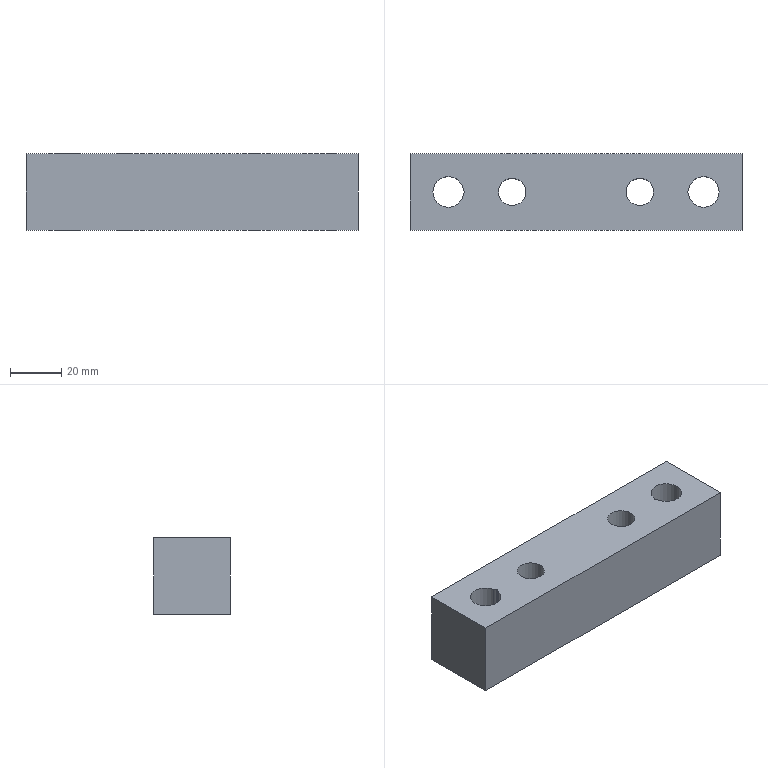Part | STEP file | YBQDJ-YL-2 | 1 solid | 16 faces | box 130 x 30 x 30 mm | volume 104775 mm3 | cylinder 10 | plane 6 | commonest cylinder face diameters 4 x4 1 x2 10.7 x2 12.01 x2
STEP:
#1=CARTESIAN_POINT('',(0.,0.,0.));
#2=DIRECTION('',(0.,0.,1.));
#3=DIRECTION('',(1.,0.,0.));
#4=AXIS2_PLACEMENT_3D('',#1,#2,#3);
#5=CARTESIAN_POINT('',(350.636,-286.292,50.));
#6=VERTEX_POINT('',#5);
#7=CARTESIAN_POINT('',(350.636,-286.292,20.));
#8=VERTEX_POINT('',#7);
#9=CARTESIAN_POINT('',(350.636,-286.292,150.));
#10=DIRECTION('',(0.,0.,-1.));
#11=VECTOR('',#10,1.);
#12=LINE('',#9,#11);
#13=CARTESIAN_POINT('',(356.5,-285.,220.));
#14=DIRECTION('',(0.,0.,-1.));
#15=DIRECTION('',(1.,0.,0.));
#16=AXIS2_PLACEMENT_3D('',#13,#14,#15);
#17=CYLINDRICAL_SURFACE('',#16,6.005);
#18=CARTESIAN_POINT('',(2.925,70.));
#19=DIRECTION('',(0.,1.));
#20=VECTOR('',#19,1.);
#21=LINE('',#18,#20);
#22=(GEOMETRIC_REPRESENTATION_CONTEXT(2)PARAMETRIC_REPRESENTATION_CONTEXT()REPRESENTATION_CONTEXT('',''));
#23=DEFINITIONAL_REPRESENTATION('',(#21),#22);
#24=PCURVE('',#17,#23);
#25=CARTESIAN_POINT('',(348.682,-286.722,150.));
#26=DIRECTION('',(0.,0.,-1.));
#27=DIRECTION('',(-1.,0.,0.));
#28=AXIS2_PLACEMENT_3D('',#25,#26,#27);
#29=CYLINDRICAL_SURFACE('',#28,2.);
#30=CARTESIAN_POINT('',(2.925,0.));
#31=DIRECTION('',(0.,1.));
#32=VECTOR('',#31,1.);
#33=LINE('',#30,#32);
#34=(GEOMETRIC_REPRESENTATION_CONTEXT(2)PARAMETRIC_REPRESENTATION_CONTEXT()REPRESENTATION_CONTEXT('',''));
#35=DEFINITIONAL_REPRESENTATION('',(#33),#34);
#36=PCURVE('',#29,#35);
#37=SURFACE_CURVE('',#12,(#24,#36),.PCURVE_S1.);
#38=EDGE_CURVE('',#6,#8,#37,.T.);
#39=ORIENTED_EDGE('',*,*,#38,.T.);
#40=CARTESIAN_POINT('',(350.636,-283.708,20.));
#41=VERTEX_POINT('',#40);
#42=CARTESIAN_POINT('',(356.5,-285.,20.));
#43=DIRECTION('',(0.,0.,1.));
#44=DIRECTION('',(1.,0.,0.));
#45=AXIS2_PLACEMENT_3D('',#42,#43,#44);
#46=CIRCLE('',#45,6.005);
#47=CARTESIAN_POINT('',(6.283,200.));
#48=DIRECTION('',(-1.,0.));
#49=VECTOR('',#48,1.);
#50=LINE('',#47,#49);
#51=(GEOMETRIC_REPRESENTATION_CONTEXT(2)PARAMETRIC_REPRESENTATION_CONTEXT()REPRESENTATION_CONTEXT('',''));
#52=DEFINITIONAL_REPRESENTATION('',(#50),#51);
#53=PCURVE('',#17,#52);
#54=CARTESIAN_POINT('',(131.5,-90.,20.));
#55=DIRECTION('',(0.,0.,1.));
#56=DIRECTION('',(0.,-1.,0.));
#57=AXIS2_PLACEMENT_3D('',#54,#55,#56);
#58=PLANE('',#57);
#59=CARTESIAN_POINT('',(195.,225.));
#60=DIRECTION('',(0.,1.));
#61=AXIS2_PLACEMENT_2D('',#59,#60);
#62=CIRCLE('',#61,6.005);
#63=(GEOMETRIC_REPRESENTATION_CONTEXT(2)PARAMETRIC_REPRESENTATION_CONTEXT()REPRESENTATION_CONTEXT('',''));
#64=DEFINITIONAL_REPRESENTATION('',(#62),#63);
#65=PCURVE('',#58,#64);
#66=SURFACE_CURVE('',#46,(#53,#65),.PCURVE_S1.);
#67=EDGE_CURVE('',#8,#41,#66,.T.);
#68=ORIENTED_EDGE('',*,*,#67,.T.);
#69=CARTESIAN_POINT('',(350.636,-283.708,50.));
#70=VERTEX_POINT('',#69);
#71=CARTESIAN_POINT('',(350.636,-283.708,150.));
#72=DIRECTION('',(0.,0.,-1.));
#73=VECTOR('',#72,1.);
#74=LINE('',#71,#73);
#75=CARTESIAN_POINT('',(-2.925,70.));
#76=DIRECTION('',(0.,1.));
#77=VECTOR('',#76,1.);
#78=LINE('',#75,#77);
#79=(GEOMETRIC_REPRESENTATION_CONTEXT(2)PARAMETRIC_REPRESENTATION_CONTEXT()REPRESENTATION_CONTEXT('',''));
#80=DEFINITIONAL_REPRESENTATION('',(#78),#79);
#81=PCURVE('',#17,#80);
#82=CARTESIAN_POINT('',(348.682,-283.278,150.));
#83=DIRECTION('',(0.,0.,-1.));
#84=DIRECTION('',(-1.,0.,0.));
#85=AXIS2_PLACEMENT_3D('',#82,#83,#84);
#86=CYLINDRICAL_SURFACE('',#85,2.);
#87=CARTESIAN_POINT('',(3.358,0.));
#88=DIRECTION('',(0.,1.));
#89=VECTOR('',#88,1.);
#90=LINE('',#87,#89);
#91=(GEOMETRIC_REPRESENTATION_CONTEXT(2)PARAMETRIC_REPRESENTATION_CONTEXT()REPRESENTATION_CONTEXT('',''));
#92=DEFINITIONAL_REPRESENTATION('',(#90),#91);
#93=PCURVE('',#86,#92);
#94=SURFACE_CURVE('',#74,(#81,#93),.PCURVE_S1.);
#95=EDGE_CURVE('',#70,#41,#94,.T.);
#96=ORIENTED_EDGE('',*,*,#95,.F.);
#97=CARTESIAN_POINT('',(356.5,-285.,50.));
#98=DIRECTION('',(0.,0.,-1.));
#99=DIRECTION('',(1.,0.,0.));
#100=AXIS2_PLACEMENT_3D('',#97,#98,#99);
#101=CIRCLE('',#100,6.005);
#102=CARTESIAN_POINT('',(-6.283,170.));
#103=DIRECTION('',(1.,0.));
#104=VECTOR('',#103,1.);
#105=LINE('',#102,#104);
#106=(GEOMETRIC_REPRESENTATION_CONTEXT(2)PARAMETRIC_REPRESENTATION_CONTEXT()REPRESENTATION_CONTEXT('',''));
#107=DEFINITIONAL_REPRESENTATION('',(#105),#106);
#108=PCURVE('',#17,#107);
#109=CARTESIAN_POINT('',(306.5,-285.,50.));
#110=DIRECTION('',(0.,0.,1.));
#111=DIRECTION('',(1.,0.,0.));
#112=AXIS2_PLACEMENT_3D('',#109,#110,#111);
#113=PLANE('',#112);
#114=CARTESIAN_POINT('',(56.005,0.));
#115=CARTESIAN_POINT('',(56.005,-10.401));
#116=CARTESIAN_POINT('',(46.998,-5.2));
#117=CARTESIAN_POINT('',(37.99,0.));
#118=CARTESIAN_POINT('',(46.998,5.2));
#119=CARTESIAN_POINT('',(56.005,10.401));
#120=CARTESIAN_POINT('',(56.005,0.));
#121=(BOUNDED_CURVE()B_SPLINE_CURVE(2,(#114,#115,#116,#117,#118,#119,#120),.UNSPECIFIED.,.T.,.F.)B_SPLINE_CURVE_WITH_KNOTS((1,2,2,2,2,1),(-2.094,0.,2.094,4.189,6.283,8.378),.UNSPECIFIED.)CURVE()GEOMETRIC_REPRESENTATION_ITEM()RATIONAL_B_SPLINE_CURVE((1.,0.5,1.,0.5,1.,0.5,1.))REPRESENTATION_ITEM(''));
#122=(GEOMETRIC_REPRESENTATION_CONTEXT(2)PARAMETRIC_REPRESENTATION_CONTEXT()REPRESENTATION_CONTEXT('',''));
#123=DEFINITIONAL_REPRESENTATION('',(#121),#122);
#124=PCURVE('',#113,#123);
#125=SURFACE_CURVE('',#101,(#108,#124),.PCURVE_S1.);
#126=EDGE_CURVE('',#70,#6,#125,.T.);
#127=ORIENTED_EDGE('',*,*,#126,.T.);
#128=EDGE_LOOP('',(#39,#68,#96,#127));
#129=FACE_BOUND('',#128,.F.);
#130=ADVANCED_FACE('',(#129),#17,.F.);
#131=CARTESIAN_POINT('',(262.364,-283.708,50.));
#132=VERTEX_POINT('',#131);
#133=CARTESIAN_POINT('',(262.364,-283.708,20.));
#134=VERTEX_POINT('',#133);
#135=CARTESIAN_POINT('',(262.364,-283.708,150.));
#136=DIRECTION('',(0.,0.,-1.));
#137=VECTOR('',#136,1.);
#138=LINE('',#135,#137);
#139=CARTESIAN_POINT('',(256.5,-285.,220.));
#140=DIRECTION('',(0.,0.,-1.));
#141=DIRECTION('',(-1.,0.,0.));
#142=AXIS2_PLACEMENT_3D('',#139,#140,#141);
#143=CYLINDRICAL_SURFACE('',#142,6.005);
#144=CARTESIAN_POINT('',(9.208,70.));
#145=DIRECTION('',(0.,1.));
#146=VECTOR('',#145,1.);
#147=LINE('',#144,#146);
#148=(GEOMETRIC_REPRESENTATION_CONTEXT(2)PARAMETRIC_REPRESENTATION_CONTEXT()REPRESENTATION_CONTEXT('',''));
#149=DEFINITIONAL_REPRESENTATION('',(#147),#148);
#150=PCURVE('',#143,#149);
#151=CARTESIAN_POINT('',(264.318,-283.278,150.));
#152=DIRECTION('',(0.,0.,-1.));
#153=DIRECTION('',(-1.,0.,0.));
#154=AXIS2_PLACEMENT_3D('',#151,#152,#153);
#155=CYLINDRICAL_SURFACE('',#154,2.);
#156=CARTESIAN_POINT('',(6.066,0.));
#157=DIRECTION('',(0.,1.));
#158=VECTOR('',#157,1.);
#159=LINE('',#156,#158);
#160=(GEOMETRIC_REPRESENTATION_CONTEXT(2)PARAMETRIC_REPRESENTATION_CONTEXT()REPRESENTATION_CONTEXT('',''));
#161=DEFINITIONAL_REPRESENTATION('',(#159),#160);
#162=PCURVE('',#155,#161);
#163=SURFACE_CURVE('',#138,(#150,#162),.PCURVE_S1.);
#164=EDGE_CURVE('',#132,#134,#163,.T.);
#165=ORIENTED_EDGE('',*,*,#164,.T.);
#166=CARTESIAN_POINT('',(262.364,-286.292,20.));
#167=VERTEX_POINT('',#166);
#168=CARTESIAN_POINT('',(256.5,-285.,20.));
#169=DIRECTION('',(0.,0.,1.));
#170=DIRECTION('',(1.,0.,0.));
#171=AXIS2_PLACEMENT_3D('',#168,#169,#170);
#172=CIRCLE('',#171,6.005);
#173=CARTESIAN_POINT('',(9.425,200.));
#174=DIRECTION('',(-1.,0.));
#175=VECTOR('',#174,1.);
#176=LINE('',#173,#175);
#177=(GEOMETRIC_REPRESENTATION_CONTEXT(2)PARAMETRIC_REPRESENTATION_CONTEXT()REPRESENTATION_CONTEXT('',''));
#178=DEFINITIONAL_REPRESENTATION('',(#176),#177);
#179=PCURVE('',#143,#178);
#180=CARTESIAN_POINT('',(195.,125.));
#181=DIRECTION('',(0.,1.));
#182=AXIS2_PLACEMENT_2D('',#180,#181);
#183=CIRCLE('',#182,6.005);
#184=(GEOMETRIC_REPRESENTATION_CONTEXT(2)PARAMETRIC_REPRESENTATION_CONTEXT()REPRESENTATION_CONTEXT('',''));
#185=DEFINITIONAL_REPRESENTATION('',(#183),#184);
#186=PCURVE('',#58,#185);
#187=SURFACE_CURVE('',#172,(#179,#186),.PCURVE_S1.);
#188=EDGE_CURVE('',#134,#167,#187,.T.);
#189=ORIENTED_EDGE('',*,*,#188,.T.);
#190=CARTESIAN_POINT('',(262.364,-286.292,50.));
#191=VERTEX_POINT('',#190);
#192=CARTESIAN_POINT('',(262.364,-286.292,150.));
#193=DIRECTION('',(0.,0.,-1.));
#194=VECTOR('',#193,1.);
#195=LINE('',#192,#194);
#196=CARTESIAN_POINT('',(3.358,70.));
#197=DIRECTION('',(0.,1.));
#198=VECTOR('',#197,1.);
#199=LINE('',#196,#198);
#200=(GEOMETRIC_REPRESENTATION_CONTEXT(2)PARAMETRIC_REPRESENTATION_CONTEXT()REPRESENTATION_CONTEXT('',''));
#201=DEFINITIONAL_REPRESENTATION('',(#199),#200);
#202=PCURVE('',#143,#201);
#203=CARTESIAN_POINT('',(264.318,-286.722,150.));
#204=DIRECTION('',(0.,0.,-1.));
#205=DIRECTION('',(-1.,0.,0.));
#206=AXIS2_PLACEMENT_3D('',#203,#204,#205);
#207=CYLINDRICAL_SURFACE('',#206,2.);
#208=CARTESIAN_POINT('',(0.2168,0.));
#209=DIRECTION('',(0.,1.));
#210=VECTOR('',#209,1.);
#211=LINE('',#208,#210);
#212=(GEOMETRIC_REPRESENTATION_CONTEXT(2)PARAMETRIC_REPRESENTATION_CONTEXT()REPRESENTATION_CONTEXT('',''));
#213=DEFINITIONAL_REPRESENTATION('',(#211),#212);
#214=PCURVE('',#207,#213);
#215=SURFACE_CURVE('',#195,(#202,#214),.PCURVE_S1.);
#216=EDGE_CURVE('',#191,#167,#215,.T.);
#217=ORIENTED_EDGE('',*,*,#216,.F.);
#218=CARTESIAN_POINT('',(256.5,-285.,50.));
#219=DIRECTION('',(0.,0.,-1.));
#220=DIRECTION('',(1.,0.,0.));
#221=AXIS2_PLACEMENT_3D('',#218,#219,#220);
#222=CIRCLE('',#221,6.005);
#223=CARTESIAN_POINT('',(3.142,170.));
#224=DIRECTION('',(1.,0.));
#225=VECTOR('',#224,1.);
#226=LINE('',#223,#225);
#227=(GEOMETRIC_REPRESENTATION_CONTEXT(2)PARAMETRIC_REPRESENTATION_CONTEXT()REPRESENTATION_CONTEXT('',''));
#228=DEFINITIONAL_REPRESENTATION('',(#226),#227);
#229=PCURVE('',#143,#228);
#230=CARTESIAN_POINT('',(-43.995,0.));
#231=CARTESIAN_POINT('',(-43.995,-10.401));
#232=CARTESIAN_POINT('',(-53.002,-5.2));
#233=CARTESIAN_POINT('',(-62.01,0.));
#234=CARTESIAN_POINT('',(-53.002,5.2));
#235=CARTESIAN_POINT('',(-43.995,10.401));
#236=CARTESIAN_POINT('',(-43.995,0.));
#237=(BOUNDED_CURVE()B_SPLINE_CURVE(2,(#230,#231,#232,#233,#234,#235,#236),.UNSPECIFIED.,.T.,.F.)B_SPLINE_CURVE_WITH_KNOTS((1,2,2,2,2,1),(-2.094,0.,2.094,4.189,6.283,8.378),.UNSPECIFIED.)CURVE()GEOMETRIC_REPRESENTATION_ITEM()RATIONAL_B_SPLINE_CURVE((1.,0.5,1.,0.5,1.,0.5,1.))REPRESENTATION_ITEM(''));
#238=(GEOMETRIC_REPRESENTATION_CONTEXT(2)PARAMETRIC_REPRESENTATION_CONTEXT()REPRESENTATION_CONTEXT('',''));
#239=DEFINITIONAL_REPRESENTATION('',(#237),#238);
#240=PCURVE('',#113,#239);
#241=SURFACE_CURVE('',#222,(#229,#240),.PCURVE_S1.);
#242=EDGE_CURVE('',#191,#132,#241,.T.);
#243=ORIENTED_EDGE('',*,*,#242,.T.);
#244=EDGE_LOOP('',(#165,#189,#217,#243));
#245=FACE_BOUND('',#244,.F.);
#246=ADVANCED_FACE('',(#245),#143,.F.);
#247=CARTESIAN_POINT('',(336.85,-285.,20.));
#248=VERTEX_POINT('',#247);
#249=CARTESIAN_POINT('',(331.5,-285.,20.));
#250=DIRECTION('',(0.,0.,1.));
#251=DIRECTION('',(1.,0.,0.));
#252=AXIS2_PLACEMENT_3D('',#249,#250,#251);
#253=CIRCLE('',#252,5.35);
#254=CARTESIAN_POINT('',(195.,200.));
#255=DIRECTION('',(0.,1.));
#256=AXIS2_PLACEMENT_2D('',#254,#255);
#257=CIRCLE('',#256,5.35);
#258=(GEOMETRIC_REPRESENTATION_CONTEXT(2)PARAMETRIC_REPRESENTATION_CONTEXT()REPRESENTATION_CONTEXT('',''));
#259=DEFINITIONAL_REPRESENTATION('',(#257),#258);
#260=PCURVE('',#58,#259);
#261=CARTESIAN_POINT('',(331.5,-285.,77.));
#262=DIRECTION('',(0.,0.,-1.));
#263=DIRECTION('',(-1.,0.,0.));
#264=AXIS2_PLACEMENT_3D('',#261,#262,#263);
#265=CYLINDRICAL_SURFACE('',#264,5.35);
#266=CARTESIAN_POINT('',(9.425,57.));
#267=DIRECTION('',(-1.,0.));
#268=VECTOR('',#267,1.);
#269=LINE('',#266,#268);
#270=(GEOMETRIC_REPRESENTATION_CONTEXT(2)PARAMETRIC_REPRESENTATION_CONTEXT()REPRESENTATION_CONTEXT('',''));
#271=DEFINITIONAL_REPRESENTATION('',(#269),#270);
#272=PCURVE('',#265,#271);
#273=SURFACE_CURVE('',#253,(#260,#272),.PCURVE_S1.);
#274=EDGE_CURVE('',#248,#248,#273,.T.);
#275=ORIENTED_EDGE('',*,*,#274,.T.);
#276=EDGE_LOOP('',(#275));
#277=FACE_BOUND('',#276,.T.);
#278=CARTESIAN_POINT('',(286.85,-285.,20.));
#279=VERTEX_POINT('',#278);
#280=CARTESIAN_POINT('',(281.5,-285.,20.));
#281=DIRECTION('',(0.,0.,-1.));
#282=DIRECTION('',(1.,0.,0.));
#283=AXIS2_PLACEMENT_3D('',#280,#281,#282);
#284=CIRCLE('',#283,5.35);
#285=CARTESIAN_POINT('',(195.,155.35));
#286=CARTESIAN_POINT('',(204.266,155.35));
#287=CARTESIAN_POINT('',(199.633,147.325));
#288=CARTESIAN_POINT('',(195.,139.3));
#289=CARTESIAN_POINT('',(190.367,147.325));
#290=CARTESIAN_POINT('',(185.734,155.35));
#291=CARTESIAN_POINT('',(195.,155.35));
#292=(BOUNDED_CURVE()B_SPLINE_CURVE(2,(#285,#286,#287,#288,#289,#290,#291),.UNSPECIFIED.,.T.,.F.)B_SPLINE_CURVE_WITH_KNOTS((1,2,2,2,2,1),(-2.094,0.,2.094,4.189,6.283,8.378),.UNSPECIFIED.)CURVE()GEOMETRIC_REPRESENTATION_ITEM()RATIONAL_B_SPLINE_CURVE((1.,0.5,1.,0.5,1.,0.5,1.))REPRESENTATION_ITEM(''));
#293=(GEOMETRIC_REPRESENTATION_CONTEXT(2)PARAMETRIC_REPRESENTATION_CONTEXT()REPRESENTATION_CONTEXT('',''));
#294=DEFINITIONAL_REPRESENTATION('',(#292),#293);
#295=PCURVE('',#58,#294);
#296=CARTESIAN_POINT('',(281.5,-285.,77.));
#297=DIRECTION('',(0.,0.,-1.));
#298=DIRECTION('',(-1.,0.,0.));
#299=AXIS2_PLACEMENT_3D('',#296,#297,#298);
#300=CYLINDRICAL_SURFACE('',#299,5.35);
#301=CARTESIAN_POINT('',(3.142,57.));
#302=DIRECTION('',(1.,0.));
#303=VECTOR('',#302,1.);
#304=LINE('',#301,#303);
#305=(GEOMETRIC_REPRESENTATION_CONTEXT(2)PARAMETRIC_REPRESENTATION_CONTEXT()REPRESENTATION_CONTEXT('',''));
#306=DEFINITIONAL_REPRESENTATION('',(#304),#305);
#307=PCURVE('',#300,#306);
#308=SURFACE_CURVE('',#284,(#295,#307),.PCURVE_S1.);
#309=EDGE_CURVE('',#279,#279,#308,.T.);
#310=ORIENTED_EDGE('',*,*,#309,.F.);
#311=EDGE_LOOP('',(#310));
#312=FACE_BOUND('',#311,.T.);
#313=ORIENTED_EDGE('',*,*,#188,.T.);
#314=CARTESIAN_POINT('',(262.868,-285.344,20.));
#315=VERTEX_POINT('',#314);
#316=CARTESIAN_POINT('',(264.318,-286.722,20.));
#317=DIRECTION('',(0.,0.,-1.));
#318=DIRECTION('',(1.,0.,0.));
#319=AXIS2_PLACEMENT_3D('',#316,#317,#318);
#320=CIRCLE('',#319,2.);
#321=CARTESIAN_POINT('',(196.722,134.818));
#322=CARTESIAN_POINT('',(200.186,134.818));
#323=CARTESIAN_POINT('',(198.454,131.818));
#324=CARTESIAN_POINT('',(196.722,128.818));
#325=CARTESIAN_POINT('',(194.99,131.818));
#326=CARTESIAN_POINT('',(193.258,134.818));
#327=CARTESIAN_POINT('',(196.722,134.818));
#328=(BOUNDED_CURVE()B_SPLINE_CURVE(2,(#321,#322,#323,#324,#325,#326,#327),.UNSPECIFIED.,.T.,.F.)B_SPLINE_CURVE_WITH_KNOTS((1,2,2,2,2,1),(-2.094,0.,2.094,4.189,6.283,8.378),.UNSPECIFIED.)CURVE()GEOMETRIC_REPRESENTATION_ITEM()RATIONAL_B_SPLINE_CURVE((1.,0.5,1.,0.5,1.,0.5,1.))REPRESENTATION_ITEM(''));
#329=(GEOMETRIC_REPRESENTATION_CONTEXT(2)PARAMETRIC_REPRESENTATION_CONTEXT()REPRESENTATION_CONTEXT('',''));
#330=DEFINITIONAL_REPRESENTATION('',(#328),#329);
#331=PCURVE('',#58,#330);
#332=CARTESIAN_POINT('',(-3.142,130.));
#333=DIRECTION('',(1.,0.));
#334=VECTOR('',#333,1.);
#335=LINE('',#332,#334);
#336=(GEOMETRIC_REPRESENTATION_CONTEXT(2)PARAMETRIC_REPRESENTATION_CONTEXT()REPRESENTATION_CONTEXT('',''));
#337=DEFINITIONAL_REPRESENTATION('',(#335),#336);
#338=PCURVE('',#207,#337);
#339=SURFACE_CURVE('',#320,(#331,#338),.PCURVE_S1.);
#340=EDGE_CURVE('',#167,#315,#339,.T.);
#341=ORIENTED_EDGE('',*,*,#340,.T.);
#342=CARTESIAN_POINT('',(262.868,-284.656,20.));
#343=VERTEX_POINT('',#342);
#344=CARTESIAN_POINT('',(262.505,-285.,20.));
#345=DIRECTION('',(0.,0.,1.));
#346=DIRECTION('',(1.,0.,0.));
#347=AXIS2_PLACEMENT_3D('',#344,#345,#346);
#348=CIRCLE('',#347,0.5);
#349=CARTESIAN_POINT('',(195.,131.005));
#350=DIRECTION('',(0.,1.));
#351=AXIS2_PLACEMENT_2D('',#349,#350);
#352=CIRCLE('',#351,0.5);
#353=(GEOMETRIC_REPRESENTATION_CONTEXT(2)PARAMETRIC_REPRESENTATION_CONTEXT()REPRESENTATION_CONTEXT('',''));
#354=DEFINITIONAL_REPRESENTATION('',(#352),#353);
#355=PCURVE('',#58,#354);
#356=CARTESIAN_POINT('',(262.505,-285.,150.));
#357=DIRECTION('',(0.,0.,-1.));
#358=DIRECTION('',(-1.,0.,0.));
#359=AXIS2_PLACEMENT_3D('',#356,#357,#358);
#360=CYLINDRICAL_SURFACE('',#359,0.5);
#361=CARTESIAN_POINT('',(9.425,130.));
#362=DIRECTION('',(-1.,0.));
#363=VECTOR('',#362,1.);
#364=LINE('',#361,#363);
#365=(GEOMETRIC_REPRESENTATION_CONTEXT(2)PARAMETRIC_REPRESENTATION_CONTEXT()REPRESENTATION_CONTEXT('',''));
#366=DEFINITIONAL_REPRESENTATION('',(#364),#365);
#367=PCURVE('',#360,#366);
#368=SURFACE_CURVE('',#348,(#355,#367),.PCURVE_S1.);
#369=EDGE_CURVE('',#315,#343,#368,.T.);
#370=ORIENTED_EDGE('',*,*,#369,.T.);
#371=CARTESIAN_POINT('',(264.318,-283.278,20.));
#372=DIRECTION('',(0.,0.,-1.));
#373=DIRECTION('',(1.,0.,0.));
#374=AXIS2_PLACEMENT_3D('',#371,#372,#373);
#375=CIRCLE('',#374,2.);
#376=CARTESIAN_POINT('',(193.278,134.818));
#377=CARTESIAN_POINT('',(196.742,134.818));
#378=CARTESIAN_POINT('',(195.01,131.818));
#379=CARTESIAN_POINT('',(193.278,128.818));
#380=CARTESIAN_POINT('',(191.546,131.818));
#381=CARTESIAN_POINT('',(189.814,134.818));
#382=CARTESIAN_POINT('',(193.278,134.818));
#383=(BOUNDED_CURVE()B_SPLINE_CURVE(2,(#376,#377,#378,#379,#380,#381,#382),.UNSPECIFIED.,.T.,.F.)B_SPLINE_CURVE_WITH_KNOTS((1,2,2,2,2,1),(-2.094,0.,2.094,4.189,6.283,8.378),.UNSPECIFIED.)CURVE()GEOMETRIC_REPRESENTATION_ITEM()RATIONAL_B_SPLINE_CURVE((1.,0.5,1.,0.5,1.,0.5,1.))REPRESENTATION_ITEM(''));
#384=(GEOMETRIC_REPRESENTATION_CONTEXT(2)PARAMETRIC_REPRESENTATION_CONTEXT()REPRESENTATION_CONTEXT('',''));
#385=DEFINITIONAL_REPRESENTATION('',(#383),#384);
#386=PCURVE('',#58,#385);
#387=CARTESIAN_POINT('',(3.142,130.));
#388=DIRECTION('',(1.,0.));
#389=VECTOR('',#388,1.);
#390=LINE('',#387,#389);
#391=(GEOMETRIC_REPRESENTATION_CONTEXT(2)PARAMETRIC_REPRESENTATION_CONTEXT()REPRESENTATION_CONTEXT('',''));
#392=DEFINITIONAL_REPRESENTATION('',(#390),#391);
#393=PCURVE('',#155,#392);
#394=SURFACE_CURVE('',#375,(#386,#393),.PCURVE_S1.);
#395=EDGE_CURVE('',#343,#134,#394,.T.);
#396=ORIENTED_EDGE('',*,*,#395,.T.);
#397=EDGE_LOOP('',(#313,#341,#370,#396));
#398=FACE_BOUND('',#397,.T.);
#399=CARTESIAN_POINT('',(241.5,-270.,20.));
#400=VERTEX_POINT('',#399);
#401=CARTESIAN_POINT('',(371.5,-270.,20.));
#402=VERTEX_POINT('',#401);
#403=CARTESIAN_POINT('',(306.5,-270.,20.));
#404=DIRECTION('',(1.,0.,0.));
#405=VECTOR('',#404,1.);
#406=LINE('',#403,#405);
#407=CARTESIAN_POINT('',(180.,175.));
#408=DIRECTION('',(0.,1.));
#409=VECTOR('',#408,1.);
#410=LINE('',#407,#409);
#411=(GEOMETRIC_REPRESENTATION_CONTEXT(2)PARAMETRIC_REPRESENTATION_CONTEXT()REPRESENTATION_CONTEXT('',''));
#412=DEFINITIONAL_REPRESENTATION('',(#410),#411);
#413=PCURVE('',#58,#412);
#414=CARTESIAN_POINT('',(306.5,-270.,40.5));
#415=DIRECTION('',(0.,-1.,0.));
#416=DIRECTION('',(0.,0.,-1.));
#417=AXIS2_PLACEMENT_3D('',#414,#415,#416);
#418=PLANE('',#417);
#419=CARTESIAN_POINT('',(20.5,0.));
#420=DIRECTION('',(0.,1.));
#421=VECTOR('',#420,1.);
#422=LINE('',#419,#421);
#423=(GEOMETRIC_REPRESENTATION_CONTEXT(2)PARAMETRIC_REPRESENTATION_CONTEXT()REPRESENTATION_CONTEXT('',''));
#424=DEFINITIONAL_REPRESENTATION('',(#422),#423);
#425=PCURVE('',#418,#424);
#426=SURFACE_CURVE('',#406,(#413,#425),.PCURVE_S1.);
#427=EDGE_CURVE('',#400,#402,#426,.T.);
#428=ORIENTED_EDGE('',*,*,#427,.T.);
#429=CARTESIAN_POINT('',(371.5,-300.,20.));
#430=VERTEX_POINT('',#429);
#431=CARTESIAN_POINT('',(371.5,-90.,20.));
#432=DIRECTION('',(0.,-1.,0.));
#433=VECTOR('',#432,1.);
#434=LINE('',#431,#433);
#435=CARTESIAN_POINT('',(0.,240.));
#436=DIRECTION('',(1.,0.));
#437=VECTOR('',#436,1.);
#438=LINE('',#435,#437);
#439=(GEOMETRIC_REPRESENTATION_CONTEXT(2)PARAMETRIC_REPRESENTATION_CONTEXT()REPRESENTATION_CONTEXT('',''));
#440=DEFINITIONAL_REPRESENTATION('',(#438),#439);
#441=PCURVE('',#58,#440);
#442=CARTESIAN_POINT('',(371.5,-90.,75.));
#443=DIRECTION('',(1.,0.,0.));
#444=DIRECTION('',(0.,0.,-1.));
#445=AXIS2_PLACEMENT_3D('',#442,#443,#444);
#446=PLANE('',#445);
#447=CARTESIAN_POINT('',(55.,0.));
#448=DIRECTION('',(0.,-1.));
#449=VECTOR('',#448,1.);
#450=LINE('',#447,#449);
#451=(GEOMETRIC_REPRESENTATION_CONTEXT(2)PARAMETRIC_REPRESENTATION_CONTEXT()REPRESENTATION_CONTEXT('',''));
#452=DEFINITIONAL_REPRESENTATION('',(#450),#451);
#453=PCURVE('',#446,#452);
#454=SURFACE_CURVE('',#434,(#441,#453),.PCURVE_S1.);
#455=EDGE_CURVE('',#402,#430,#454,.T.);
#456=ORIENTED_EDGE('',*,*,#455,.T.);
#457=CARTESIAN_POINT('',(241.5,-300.,20.));
#458=VERTEX_POINT('',#457);
#459=CARTESIAN_POINT('',(131.5,-300.,20.));
#460=DIRECTION('',(-1.,0.,0.));
#461=VECTOR('',#460,1.);
#462=LINE('',#459,#461);
#463=CARTESIAN_POINT('',(210.,0.));
#464=DIRECTION('',(0.,-1.));
#465=VECTOR('',#464,1.);
#466=LINE('',#463,#465);
#467=(GEOMETRIC_REPRESENTATION_CONTEXT(2)PARAMETRIC_REPRESENTATION_CONTEXT()REPRESENTATION_CONTEXT('',''));
#468=DEFINITIONAL_REPRESENTATION('',(#466),#467);
#469=PCURVE('',#58,#468);
#470=CARTESIAN_POINT('',(131.5,-300.,75.));
#471=DIRECTION('',(0.,-1.,0.));
#472=DIRECTION('',(0.,0.,-1.));
#473=AXIS2_PLACEMENT_3D('',#470,#471,#472);
#474=PLANE('',#473);
#475=CARTESIAN_POINT('',(55.,0.));
#476=DIRECTION('',(0.,-1.));
#477=VECTOR('',#476,1.);
#478=LINE('',#475,#477);
#479=(GEOMETRIC_REPRESENTATION_CONTEXT(2)PARAMETRIC_REPRESENTATION_CONTEXT()REPRESENTATION_CONTEXT('',''));
#480=DEFINITIONAL_REPRESENTATION('',(#478),#479);
#481=PCURVE('',#474,#480);
#482=SURFACE_CURVE('',#462,(#469,#481),.PCURVE_S1.);
#483=EDGE_CURVE('',#430,#458,#482,.T.);
#484=ORIENTED_EDGE('',*,*,#483,.T.);
#485=CARTESIAN_POINT('',(241.5,-90.,20.));
#486=DIRECTION('',(0.,-1.,0.));
#487=VECTOR('',#486,1.);
#488=LINE('',#485,#487);
#489=CARTESIAN_POINT('',(0.,110.));
#490=DIRECTION('',(1.,0.));
#491=VECTOR('',#490,1.);
#492=LINE('',#489,#491);
#493=(GEOMETRIC_REPRESENTATION_CONTEXT(2)PARAMETRIC_REPRESENTATION_CONTEXT()REPRESENTATION_CONTEXT('',''));
#494=DEFINITIONAL_REPRESENTATION('',(#492),#493);
#495=PCURVE('',#58,#494);
#496=CARTESIAN_POINT('',(241.5,-90.,75.));
#497=DIRECTION('',(1.,0.,0.));
#498=DIRECTION('',(0.,0.,-1.));
#499=AXIS2_PLACEMENT_3D('',#496,#497,#498);
#500=PLANE('',#499);
#501=CARTESIAN_POINT('',(55.,0.));
#502=DIRECTION('',(0.,-1.));
#503=VECTOR('',#502,1.);
#504=LINE('',#501,#503);
#505=(GEOMETRIC_REPRESENTATION_CONTEXT(2)PARAMETRIC_REPRESENTATION_CONTEXT()REPRESENTATION_CONTEXT('',''));
#506=DEFINITIONAL_REPRESENTATION('',(#504),#505);
#507=PCURVE('',#500,#506);
#508=SURFACE_CURVE('',#488,(#495,#507),.PCURVE_S1.);
#509=EDGE_CURVE('',#400,#458,#508,.T.);
#510=ORIENTED_EDGE('',*,*,#509,.F.);
#511=EDGE_LOOP('',(#428,#456,#484,#510));
#512=FACE_BOUND('',#511,.T.);
#513=CARTESIAN_POINT('',(350.132,-284.656,20.));
#514=VERTEX_POINT('',#513);
#515=CARTESIAN_POINT('',(348.682,-283.278,20.));
#516=DIRECTION('',(0.,0.,1.));
#517=DIRECTION('',(1.,0.,0.));
#518=AXIS2_PLACEMENT_3D('',#515,#516,#517);
#519=CIRCLE('',#518,2.);
#520=CARTESIAN_POINT('',(193.278,217.182));
#521=DIRECTION('',(0.,1.));
#522=AXIS2_PLACEMENT_2D('',#520,#521);
#523=CIRCLE('',#522,2.);
#524=(GEOMETRIC_REPRESENTATION_CONTEXT(2)PARAMETRIC_REPRESENTATION_CONTEXT()REPRESENTATION_CONTEXT('',''));
#525=DEFINITIONAL_REPRESENTATION('',(#523),#524);
#526=PCURVE('',#58,#525);
#527=CARTESIAN_POINT('',(9.425,130.));
#528=DIRECTION('',(-1.,0.));
#529=VECTOR('',#528,1.);
#530=LINE('',#527,#529);
#531=(GEOMETRIC_REPRESENTATION_CONTEXT(2)PARAMETRIC_REPRESENTATION_CONTEXT()REPRESENTATION_CONTEXT('',''));
#532=DEFINITIONAL_REPRESENTATION('',(#530),#531);
#533=PCURVE('',#86,#532);
#534=SURFACE_CURVE('',#519,(#526,#533),.PCURVE_S1.);
#535=EDGE_CURVE('',#514,#41,#534,.T.);
#536=ORIENTED_EDGE('',*,*,#535,.F.);
#537=CARTESIAN_POINT('',(350.132,-285.344,20.));
#538=VERTEX_POINT('',#537);
#539=CARTESIAN_POINT('',(350.495,-285.,20.));
#540=DIRECTION('',(0.,0.,-1.));
#541=DIRECTION('',(1.,0.,0.));
#542=AXIS2_PLACEMENT_3D('',#539,#540,#541);
#543=CIRCLE('',#542,0.5);
#544=CARTESIAN_POINT('',(195.,219.495));
#545=CARTESIAN_POINT('',(195.866,219.495));
#546=CARTESIAN_POINT('',(195.433,218.745));
#547=CARTESIAN_POINT('',(195.,217.995));
#548=CARTESIAN_POINT('',(194.567,218.745));
#549=CARTESIAN_POINT('',(194.134,219.495));
#550=CARTESIAN_POINT('',(195.,219.495));
#551=(BOUNDED_CURVE()B_SPLINE_CURVE(2,(#544,#545,#546,#547,#548,#549,#550),.UNSPECIFIED.,.T.,.F.)B_SPLINE_CURVE_WITH_KNOTS((1,2,2,2,2,1),(-2.094,0.,2.094,4.189,6.283,8.378),.UNSPECIFIED.)CURVE()GEOMETRIC_REPRESENTATION_ITEM()RATIONAL_B_SPLINE_CURVE((1.,0.5,1.,0.5,1.,0.5,1.))REPRESENTATION_ITEM(''));
#552=(GEOMETRIC_REPRESENTATION_CONTEXT(2)PARAMETRIC_REPRESENTATION_CONTEXT()REPRESENTATION_CONTEXT('',''));
#553=DEFINITIONAL_REPRESENTATION('',(#551),#552);
#554=PCURVE('',#58,#553);
#555=CARTESIAN_POINT('',(350.495,-285.,150.));
#556=DIRECTION('',(0.,0.,-1.));
#557=DIRECTION('',(-1.,0.,0.));
#558=AXIS2_PLACEMENT_3D('',#555,#556,#557);
#559=CYLINDRICAL_SURFACE('',#558,0.5);
#560=CARTESIAN_POINT('',(-3.142,130.));
#561=DIRECTION('',(1.,0.));
#562=VECTOR('',#561,1.);
#563=LINE('',#560,#562);
#564=(GEOMETRIC_REPRESENTATION_CONTEXT(2)PARAMETRIC_REPRESENTATION_CONTEXT()REPRESENTATION_CONTEXT('',''));
#565=DEFINITIONAL_REPRESENTATION('',(#563),#564);
#566=PCURVE('',#559,#565);
#567=SURFACE_CURVE('',#543,(#554,#566),.PCURVE_S1.);
#568=EDGE_CURVE('',#538,#514,#567,.T.);
#569=ORIENTED_EDGE('',*,*,#568,.F.);
#570=CARTESIAN_POINT('',(348.682,-286.722,20.));
#571=DIRECTION('',(0.,0.,1.));
#572=DIRECTION('',(1.,0.,0.));
#573=AXIS2_PLACEMENT_3D('',#570,#571,#572);
#574=CIRCLE('',#573,2.);
#575=CARTESIAN_POINT('',(196.722,217.182));
#576=DIRECTION('',(0.,1.));
#577=AXIS2_PLACEMENT_2D('',#575,#576);
#578=CIRCLE('',#577,2.);
#579=(GEOMETRIC_REPRESENTATION_CONTEXT(2)PARAMETRIC_REPRESENTATION_CONTEXT()REPRESENTATION_CONTEXT('',''));
#580=DEFINITIONAL_REPRESENTATION('',(#578),#579);
#581=PCURVE('',#58,#580);
#582=CARTESIAN_POINT('',(3.142,130.));
#583=DIRECTION('',(-1.,0.));
#584=VECTOR('',#583,1.);
#585=LINE('',#582,#584);
#586=(GEOMETRIC_REPRESENTATION_CONTEXT(2)PARAMETRIC_REPRESENTATION_CONTEXT()REPRESENTATION_CONTEXT('',''));
#587=DEFINITIONAL_REPRESENTATION('',(#585),#586);
#588=PCURVE('',#29,#587);
#589=SURFACE_CURVE('',#574,(#581,#588),.PCURVE_S1.);
#590=EDGE_CURVE('',#8,#538,#589,.T.);
#591=ORIENTED_EDGE('',*,*,#590,.F.);
#592=ORIENTED_EDGE('',*,*,#67,.T.);
#593=EDGE_LOOP('',(#536,#569,#591,#592));
#594=FACE_BOUND('',#593,.T.);
#595=ADVANCED_FACE('',(#277,#312,#398,#512,#594),#58,.F.);
#596=CARTESIAN_POINT('',(336.85,-285.,50.));
#597=VERTEX_POINT('',#596);
#598=CARTESIAN_POINT('',(331.5,-285.,50.));
#599=DIRECTION('',(0.,0.,-1.));
#600=DIRECTION('',(1.,0.,0.));
#601=AXIS2_PLACEMENT_3D('',#598,#599,#600);
#602=CIRCLE('',#601,5.35);
#603=CARTESIAN_POINT('',(30.35,0.));
#604=CARTESIAN_POINT('',(30.35,-9.266));
#605=CARTESIAN_POINT('',(22.325,-4.633));
#606=CARTESIAN_POINT('',(14.3,0.));
#607=CARTESIAN_POINT('',(22.325,4.633));
#608=CARTESIAN_POINT('',(30.35,9.266));
#609=CARTESIAN_POINT('',(30.35,0.));
#610=(BOUNDED_CURVE()B_SPLINE_CURVE(2,(#603,#604,#605,#606,#607,#608,#609),.UNSPECIFIED.,.T.,.F.)B_SPLINE_CURVE_WITH_KNOTS((1,2,2,2,2,1),(-2.094,0.,2.094,4.189,6.283,8.378),.UNSPECIFIED.)CURVE()GEOMETRIC_REPRESENTATION_ITEM()RATIONAL_B_SPLINE_CURVE((1.,0.5,1.,0.5,1.,0.5,1.))REPRESENTATION_ITEM(''));
#611=(GEOMETRIC_REPRESENTATION_CONTEXT(2)PARAMETRIC_REPRESENTATION_CONTEXT()REPRESENTATION_CONTEXT('',''));
#612=DEFINITIONAL_REPRESENTATION('',(#610),#611);
#613=PCURVE('',#113,#612);
#614=CARTESIAN_POINT('',(3.142,27.));
#615=DIRECTION('',(1.,0.));
#616=VECTOR('',#615,1.);
#617=LINE('',#614,#616);
#618=(GEOMETRIC_REPRESENTATION_CONTEXT(2)PARAMETRIC_REPRESENTATION_CONTEXT()REPRESENTATION_CONTEXT('',''));
#619=DEFINITIONAL_REPRESENTATION('',(#617),#618);
#620=PCURVE('',#265,#619);
#621=SURFACE_CURVE('',#602,(#613,#620),.PCURVE_S1.);
#622=EDGE_CURVE('',#597,#597,#621,.T.);
#623=ORIENTED_EDGE('',*,*,#622,.T.);
#624=EDGE_LOOP('',(#623));
#625=FACE_BOUND('',#624,.T.);
#626=CARTESIAN_POINT('',(286.85,-285.,50.));
#627=VERTEX_POINT('',#626);
#628=CARTESIAN_POINT('',(281.5,-285.,50.));
#629=DIRECTION('',(0.,0.,1.));
#630=DIRECTION('',(1.,0.,0.));
#631=AXIS2_PLACEMENT_3D('',#628,#629,#630);
#632=CIRCLE('',#631,5.35);
#633=CARTESIAN_POINT('',(-25.,0.));
#634=DIRECTION('',(1.,0.));
#635=AXIS2_PLACEMENT_2D('',#633,#634);
#636=CIRCLE('',#635,5.35);
#637=(GEOMETRIC_REPRESENTATION_CONTEXT(2)PARAMETRIC_REPRESENTATION_CONTEXT()REPRESENTATION_CONTEXT('',''));
#638=DEFINITIONAL_REPRESENTATION('',(#636),#637);
#639=PCURVE('',#113,#638);
#640=CARTESIAN_POINT('',(9.425,27.));
#641=DIRECTION('',(-1.,0.));
#642=VECTOR('',#641,1.);
#643=LINE('',#640,#642);
#644=(GEOMETRIC_REPRESENTATION_CONTEXT(2)PARAMETRIC_REPRESENTATION_CONTEXT()REPRESENTATION_CONTEXT('',''));
#645=DEFINITIONAL_REPRESENTATION('',(#643),#644);
#646=PCURVE('',#300,#645);
#647=SURFACE_CURVE('',#632,(#639,#646),.PCURVE_S1.);
#648=EDGE_CURVE('',#627,#627,#647,.T.);
#649=ORIENTED_EDGE('',*,*,#648,.F.);
#650=EDGE_LOOP('',(#649));
#651=FACE_BOUND('',#650,.T.);
#652=CARTESIAN_POINT('',(262.868,-284.656,50.));
#653=VERTEX_POINT('',#652);
#654=CARTESIAN_POINT('',(262.868,-285.344,50.));
#655=VERTEX_POINT('',#654);
#656=CARTESIAN_POINT('',(262.505,-285.,50.));
#657=DIRECTION('',(0.,0.,-1.));
#658=DIRECTION('',(1.,0.,0.));
#659=AXIS2_PLACEMENT_3D('',#656,#657,#658);
#660=CIRCLE('',#659,0.5);
#661=CARTESIAN_POINT('',(-43.495,0.));
#662=CARTESIAN_POINT('',(-43.495,-0.866));
#663=CARTESIAN_POINT('',(-44.245,-0.433));
#664=CARTESIAN_POINT('',(-44.995,0.));
#665=CARTESIAN_POINT('',(-44.245,0.433));
#666=CARTESIAN_POINT('',(-43.495,0.866));
#667=CARTESIAN_POINT('',(-43.495,0.));
#668=(BOUNDED_CURVE()B_SPLINE_CURVE(2,(#661,#662,#663,#664,#665,#666,#667),.UNSPECIFIED.,.T.,.F.)B_SPLINE_CURVE_WITH_KNOTS((1,2,2,2,2,1),(-2.094,0.,2.094,4.189,6.283,8.378),.UNSPECIFIED.)CURVE()GEOMETRIC_REPRESENTATION_ITEM()RATIONAL_B_SPLINE_CURVE((1.,0.5,1.,0.5,1.,0.5,1.))REPRESENTATION_ITEM(''));
#669=(GEOMETRIC_REPRESENTATION_CONTEXT(2)PARAMETRIC_REPRESENTATION_CONTEXT()REPRESENTATION_CONTEXT('',''));
#670=DEFINITIONAL_REPRESENTATION('',(#668),#669);
#671=PCURVE('',#113,#670);
#672=CARTESIAN_POINT('',(-3.142,100.));
#673=DIRECTION('',(1.,0.));
#674=VECTOR('',#673,1.);
#675=LINE('',#672,#674);
#676=(GEOMETRIC_REPRESENTATION_CONTEXT(2)PARAMETRIC_REPRESENTATION_CONTEXT()REPRESENTATION_CONTEXT('',''));
#677=DEFINITIONAL_REPRESENTATION('',(#675),#676);
#678=PCURVE('',#360,#677);
#679=SURFACE_CURVE('',#660,(#671,#678),.PCURVE_S1.);
#680=EDGE_CURVE('',#653,#655,#679,.T.);
#681=ORIENTED_EDGE('',*,*,#680,.T.);
#682=CARTESIAN_POINT('',(264.318,-286.722,50.));
#683=DIRECTION('',(0.,0.,1.));
#684=DIRECTION('',(1.,0.,0.));
#685=AXIS2_PLACEMENT_3D('',#682,#683,#684);
#686=CIRCLE('',#685,2.);
#687=CARTESIAN_POINT('',(-42.182,-1.722));
#688=DIRECTION('',(1.,0.));
#689=AXIS2_PLACEMENT_2D('',#687,#688);
#690=CIRCLE('',#689,2.);
#691=(GEOMETRIC_REPRESENTATION_CONTEXT(2)PARAMETRIC_REPRESENTATION_CONTEXT()REPRESENTATION_CONTEXT('',''));
#692=DEFINITIONAL_REPRESENTATION('',(#690),#691);
#693=PCURVE('',#113,#692);
#694=CARTESIAN_POINT('',(3.142,100.));
#695=DIRECTION('',(-1.,0.));
#696=VECTOR('',#695,1.);
#697=LINE('',#694,#696);
#698=(GEOMETRIC_REPRESENTATION_CONTEXT(2)PARAMETRIC_REPRESENTATION_CONTEXT()REPRESENTATION_CONTEXT('',''));
#699=DEFINITIONAL_REPRESENTATION('',(#697),#698);
#700=PCURVE('',#207,#699);
#701=SURFACE_CURVE('',#686,(#693,#700),.PCURVE_S1.);
#702=EDGE_CURVE('',#655,#191,#701,.T.);
#703=ORIENTED_EDGE('',*,*,#702,.T.);
#704=ORIENTED_EDGE('',*,*,#242,.T.);
#705=CARTESIAN_POINT('',(264.318,-283.278,50.));
#706=DIRECTION('',(0.,0.,1.));
#707=DIRECTION('',(1.,0.,0.));
#708=AXIS2_PLACEMENT_3D('',#705,#706,#707);
#709=CIRCLE('',#708,2.);
#710=CARTESIAN_POINT('',(-42.182,1.722));
#711=DIRECTION('',(1.,0.));
#712=AXIS2_PLACEMENT_2D('',#710,#711);
#713=CIRCLE('',#712,2.);
#714=(GEOMETRIC_REPRESENTATION_CONTEXT(2)PARAMETRIC_REPRESENTATION_CONTEXT()REPRESENTATION_CONTEXT('',''));
#715=DEFINITIONAL_REPRESENTATION('',(#713),#714);
#716=PCURVE('',#113,#715);
#717=CARTESIAN_POINT('',(9.425,100.));
#718=DIRECTION('',(-1.,0.));
#719=VECTOR('',#718,1.);
#720=LINE('',#717,#719);
#721=(GEOMETRIC_REPRESENTATION_CONTEXT(2)PARAMETRIC_REPRESENTATION_CONTEXT()REPRESENTATION_CONTEXT('',''));
#722=DEFINITIONAL_REPRESENTATION('',(#720),#721);
#723=PCURVE('',#155,#722);
#724=SURFACE_CURVE('',#709,(#716,#723),.PCURVE_S1.);
#725=EDGE_CURVE('',#132,#653,#724,.T.);
#726=ORIENTED_EDGE('',*,*,#725,.T.);
#727=EDGE_LOOP('',(#681,#703,#704,#726));
#728=FACE_BOUND('',#727,.T.);
#729=CARTESIAN_POINT('',(371.5,-300.,50.));
#730=VERTEX_POINT('',#729);
#731=CARTESIAN_POINT('',(241.5,-300.,50.));
#732=VERTEX_POINT('',#731);
#733=CARTESIAN_POINT('',(131.5,-300.,50.));
#734=DIRECTION('',(-1.,0.,0.));
#735=VECTOR('',#734,1.);
#736=LINE('',#733,#735);
#737=CARTESIAN_POINT('',(-175.,-15.));
#738=DIRECTION('',(-1.,0.));
#739=VECTOR('',#738,1.);
#740=LINE('',#737,#739);
#741=(GEOMETRIC_REPRESENTATION_CONTEXT(2)PARAMETRIC_REPRESENTATION_CONTEXT()REPRESENTATION_CONTEXT('',''));
#742=DEFINITIONAL_REPRESENTATION('',(#740),#741);
#743=PCURVE('',#113,#742);
#744=CARTESIAN_POINT('',(25.,0.));
#745=DIRECTION('',(0.,-1.));
#746=VECTOR('',#745,1.);
#747=LINE('',#744,#746);
#748=(GEOMETRIC_REPRESENTATION_CONTEXT(2)PARAMETRIC_REPRESENTATION_CONTEXT()REPRESENTATION_CONTEXT('',''));
#749=DEFINITIONAL_REPRESENTATION('',(#747),#748);
#750=PCURVE('',#474,#749);
#751=SURFACE_CURVE('',#736,(#743,#750),.PCURVE_S1.);
#752=EDGE_CURVE('',#730,#732,#751,.T.);
#753=ORIENTED_EDGE('',*,*,#752,.F.);
#754=CARTESIAN_POINT('',(371.5,-270.,50.));
#755=VERTEX_POINT('',#754);
#756=CARTESIAN_POINT('',(371.5,-90.,50.));
#757=DIRECTION('',(0.,-1.,0.));
#758=VECTOR('',#757,1.);
#759=LINE('',#756,#758);
#760=CARTESIAN_POINT('',(65.,195.));
#761=DIRECTION('',(0.,-1.));
#762=VECTOR('',#761,1.);
#763=LINE('',#760,#762);
#764=(GEOMETRIC_REPRESENTATION_CONTEXT(2)PARAMETRIC_REPRESENTATION_CONTEXT()REPRESENTATION_CONTEXT('',''));
#765=DEFINITIONAL_REPRESENTATION('',(#763),#764);
#766=PCURVE('',#113,#765);
#767=CARTESIAN_POINT('',(25.,0.));
#768=DIRECTION('',(0.,-1.));
#769=VECTOR('',#768,1.);
#770=LINE('',#767,#769);
#771=(GEOMETRIC_REPRESENTATION_CONTEXT(2)PARAMETRIC_REPRESENTATION_CONTEXT()REPRESENTATION_CONTEXT('',''));
#772=DEFINITIONAL_REPRESENTATION('',(#770),#771);
#773=PCURVE('',#446,#772);
#774=SURFACE_CURVE('',#759,(#766,#773),.PCURVE_S1.);
#775=EDGE_CURVE('',#755,#730,#774,.T.);
#776=ORIENTED_EDGE('',*,*,#775,.F.);
#777=CARTESIAN_POINT('',(241.5,-270.,50.));
#778=VERTEX_POINT('',#777);
#779=CARTESIAN_POINT('',(306.5,-270.,50.));
#780=DIRECTION('',(-1.,0.,0.));
#781=VECTOR('',#780,1.);
#782=LINE('',#779,#781);
#783=CARTESIAN_POINT('',(0.,15.));
#784=DIRECTION('',(-1.,0.));
#785=VECTOR('',#784,1.);
#786=LINE('',#783,#785);
#787=(GEOMETRIC_REPRESENTATION_CONTEXT(2)PARAMETRIC_REPRESENTATION_CONTEXT()REPRESENTATION_CONTEXT('',''));
#788=DEFINITIONAL_REPRESENTATION('',(#786),#787);
#789=PCURVE('',#113,#788);
#790=CARTESIAN_POINT('',(-9.5,0.));
#791=DIRECTION('',(0.,-1.));
#792=VECTOR('',#791,1.);
#793=LINE('',#790,#792);
#794=(GEOMETRIC_REPRESENTATION_CONTEXT(2)PARAMETRIC_REPRESENTATION_CONTEXT()REPRESENTATION_CONTEXT('',''));
#795=DEFINITIONAL_REPRESENTATION('',(#793),#794);
#796=PCURVE('',#418,#795);
#797=SURFACE_CURVE('',#782,(#789,#796),.PCURVE_S1.);
#798=EDGE_CURVE('',#755,#778,#797,.T.);
#799=ORIENTED_EDGE('',*,*,#798,.T.);
#800=CARTESIAN_POINT('',(241.5,-285.,50.));
#801=DIRECTION('',(0.,1.,0.));
#802=VECTOR('',#801,1.);
#803=LINE('',#800,#802);
#804=CARTESIAN_POINT('',(-65.,0.));
#805=DIRECTION('',(0.,1.));
#806=VECTOR('',#805,1.);
#807=LINE('',#804,#806);
#808=(GEOMETRIC_REPRESENTATION_CONTEXT(2)PARAMETRIC_REPRESENTATION_CONTEXT()REPRESENTATION_CONTEXT('',''));
#809=DEFINITIONAL_REPRESENTATION('',(#807),#808);
#810=PCURVE('',#113,#809);
#811=CARTESIAN_POINT('',(25.,-195.));
#812=DIRECTION('',(0.,1.));
#813=VECTOR('',#812,1.);
#814=LINE('',#811,#813);
#815=(GEOMETRIC_REPRESENTATION_CONTEXT(2)PARAMETRIC_REPRESENTATION_CONTEXT()REPRESENTATION_CONTEXT('',''));
#816=DEFINITIONAL_REPRESENTATION('',(#814),#815);
#817=PCURVE('',#500,#816);
#818=SURFACE_CURVE('',#803,(#810,#817),.PCURVE_S1.);
#819=EDGE_CURVE('',#732,#778,#818,.T.);
#820=ORIENTED_EDGE('',*,*,#819,.F.);
#821=EDGE_LOOP('',(#753,#776,#799,#820));
#822=FACE_BOUND('',#821,.T.);
#823=CARTESIAN_POINT('',(350.132,-284.656,50.));
#824=VERTEX_POINT('',#823);
#825=CARTESIAN_POINT('',(348.682,-283.278,50.));
#826=DIRECTION('',(0.,0.,-1.));
#827=DIRECTION('',(1.,0.,0.));
#828=AXIS2_PLACEMENT_3D('',#825,#826,#827);
#829=CIRCLE('',#828,2.);
#830=CARTESIAN_POINT('',(44.182,1.722));
#831=CARTESIAN_POINT('',(44.182,-1.742));
#832=CARTESIAN_POINT('',(41.182,-0.01034));
#833=CARTESIAN_POINT('',(38.182,1.722));
#834=CARTESIAN_POINT('',(41.182,3.454));
#835=CARTESIAN_POINT('',(44.182,5.186));
#836=CARTESIAN_POINT('',(44.182,1.722));
#837=(BOUNDED_CURVE()B_SPLINE_CURVE(2,(#830,#831,#832,#833,#834,#835,#836),.UNSPECIFIED.,.T.,.F.)B_SPLINE_CURVE_WITH_KNOTS((1,2,2,2,2,1),(-2.094,0.,2.094,4.189,6.283,8.378),.UNSPECIFIED.)CURVE()GEOMETRIC_REPRESENTATION_ITEM()RATIONAL_B_SPLINE_CURVE((1.,0.5,1.,0.5,1.,0.5,1.))REPRESENTATION_ITEM(''));
#838=(GEOMETRIC_REPRESENTATION_CONTEXT(2)PARAMETRIC_REPRESENTATION_CONTEXT()REPRESENTATION_CONTEXT('',''));
#839=DEFINITIONAL_REPRESENTATION('',(#837),#838);
#840=PCURVE('',#113,#839);
#841=CARTESIAN_POINT('',(3.142,100.));
#842=DIRECTION('',(1.,0.));
#843=VECTOR('',#842,1.);
#844=LINE('',#841,#843);
#845=(GEOMETRIC_REPRESENTATION_CONTEXT(2)PARAMETRIC_REPRESENTATION_CONTEXT()REPRESENTATION_CONTEXT('',''));
#846=DEFINITIONAL_REPRESENTATION('',(#844),#845);
#847=PCURVE('',#86,#846);
#848=SURFACE_CURVE('',#829,(#840,#847),.PCURVE_S1.);
#849=EDGE_CURVE('',#70,#824,#848,.T.);
#850=ORIENTED_EDGE('',*,*,#849,.F.);
#851=ORIENTED_EDGE('',*,*,#126,.T.);
#852=CARTESIAN_POINT('',(350.132,-285.344,50.));
#853=VERTEX_POINT('',#852);
#854=CARTESIAN_POINT('',(348.682,-286.722,50.));
#855=DIRECTION('',(0.,0.,-1.));
#856=DIRECTION('',(1.,0.,0.));
#857=AXIS2_PLACEMENT_3D('',#854,#855,#856);
#858=CIRCLE('',#857,2.);
#859=CARTESIAN_POINT('',(44.182,-1.722));
#860=CARTESIAN_POINT('',(44.182,-5.186));
#861=CARTESIAN_POINT('',(41.182,-3.454));
#862=CARTESIAN_POINT('',(38.182,-1.722));
#863=CARTESIAN_POINT('',(41.182,0.01034));
#864=CARTESIAN_POINT('',(44.182,1.742));
#865=CARTESIAN_POINT('',(44.182,-1.722));
#866=(BOUNDED_CURVE()B_SPLINE_CURVE(2,(#859,#860,#861,#862,#863,#864,#865),.UNSPECIFIED.,.T.,.F.)B_SPLINE_CURVE_WITH_KNOTS((1,2,2,2,2,1),(-2.094,0.,2.094,4.189,6.283,8.378),.UNSPECIFIED.)CURVE()GEOMETRIC_REPRESENTATION_ITEM()RATIONAL_B_SPLINE_CURVE((1.,0.5,1.,0.5,1.,0.5,1.))REPRESENTATION_ITEM(''));
#867=(GEOMETRIC_REPRESENTATION_CONTEXT(2)PARAMETRIC_REPRESENTATION_CONTEXT()REPRESENTATION_CONTEXT('',''));
#868=DEFINITIONAL_REPRESENTATION('',(#866),#867);
#869=PCURVE('',#113,#868);
#870=CARTESIAN_POINT('',(-3.142,100.));
#871=DIRECTION('',(1.,0.));
#872=VECTOR('',#871,1.);
#873=LINE('',#870,#872);
#874=(GEOMETRIC_REPRESENTATION_CONTEXT(2)PARAMETRIC_REPRESENTATION_CONTEXT()REPRESENTATION_CONTEXT('',''));
#875=DEFINITIONAL_REPRESENTATION('',(#873),#874);
#876=PCURVE('',#29,#875);
#877=SURFACE_CURVE('',#858,(#869,#876),.PCURVE_S1.);
#878=EDGE_CURVE('',#853,#6,#877,.T.);
#879=ORIENTED_EDGE('',*,*,#878,.F.);
#880=CARTESIAN_POINT('',(350.495,-285.,50.));
#881=DIRECTION('',(0.,0.,1.));
#882=DIRECTION('',(1.,0.,0.));
#883=AXIS2_PLACEMENT_3D('',#880,#881,#882);
#884=CIRCLE('',#883,0.5);
#885=CARTESIAN_POINT('',(43.995,0.));
#886=DIRECTION('',(1.,0.));
#887=AXIS2_PLACEMENT_2D('',#885,#886);
#888=CIRCLE('',#887,0.5);
#889=(GEOMETRIC_REPRESENTATION_CONTEXT(2)PARAMETRIC_REPRESENTATION_CONTEXT()REPRESENTATION_CONTEXT('',''));
#890=DEFINITIONAL_REPRESENTATION('',(#888),#889);
#891=PCURVE('',#113,#890);
#892=CARTESIAN_POINT('',(3.142,100.));
#893=DIRECTION('',(-1.,0.));
#894=VECTOR('',#893,1.);
#895=LINE('',#892,#894);
#896=(GEOMETRIC_REPRESENTATION_CONTEXT(2)PARAMETRIC_REPRESENTATION_CONTEXT()REPRESENTATION_CONTEXT('',''));
#897=DEFINITIONAL_REPRESENTATION('',(#895),#896);
#898=PCURVE('',#559,#897);
#899=SURFACE_CURVE('',#884,(#891,#898),.PCURVE_S1.);
#900=EDGE_CURVE('',#824,#853,#899,.T.);
#901=ORIENTED_EDGE('',*,*,#900,.F.);
#902=EDGE_LOOP('',(#850,#851,#879,#901));
#903=FACE_BOUND('',#902,.T.);
#904=ADVANCED_FACE('',(#625,#651,#728,#822,#903),#113,.T.);
#905=CARTESIAN_POINT('',(371.5,-300.,75.));
#906=DIRECTION('',(0.,0.,-1.));
#907=VECTOR('',#906,1.);
#908=LINE('',#905,#907);
#909=CARTESIAN_POINT('',(0.,240.));
#910=DIRECTION('',(1.,0.));
#911=VECTOR('',#910,1.);
#912=LINE('',#909,#911);
#913=(GEOMETRIC_REPRESENTATION_CONTEXT(2)PARAMETRIC_REPRESENTATION_CONTEXT()REPRESENTATION_CONTEXT('',''));
#914=DEFINITIONAL_REPRESENTATION('',(#912),#913);
#915=PCURVE('',#474,#914);
#916=CARTESIAN_POINT('',(0.,-210.));
#917=DIRECTION('',(1.,0.));
#918=VECTOR('',#917,1.);
#919=LINE('',#916,#918);
#920=(GEOMETRIC_REPRESENTATION_CONTEXT(2)PARAMETRIC_REPRESENTATION_CONTEXT()REPRESENTATION_CONTEXT('',''));
#921=DEFINITIONAL_REPRESENTATION('',(#919),#920);
#922=PCURVE('',#446,#921);
#923=SURFACE_CURVE('',#908,(#915,#922),.PCURVE_S1.);
#924=EDGE_CURVE('',#730,#430,#923,.T.);
#925=ORIENTED_EDGE('',*,*,#924,.F.);
#926=ORIENTED_EDGE('',*,*,#752,.T.);
#927=CARTESIAN_POINT('',(241.5,-300.,75.));
#928=DIRECTION('',(0.,0.,-1.));
#929=VECTOR('',#928,1.);
#930=LINE('',#927,#929);
#931=CARTESIAN_POINT('',(0.,110.));
#932=DIRECTION('',(1.,0.));
#933=VECTOR('',#932,1.);
#934=LINE('',#931,#933);
#935=(GEOMETRIC_REPRESENTATION_CONTEXT(2)PARAMETRIC_REPRESENTATION_CONTEXT()REPRESENTATION_CONTEXT('',''));
#936=DEFINITIONAL_REPRESENTATION('',(#934),#935);
#937=PCURVE('',#474,#936);
#938=CARTESIAN_POINT('',(0.,-210.));
#939=DIRECTION('',(1.,0.));
#940=VECTOR('',#939,1.);
#941=LINE('',#938,#940);
#942=(GEOMETRIC_REPRESENTATION_CONTEXT(2)PARAMETRIC_REPRESENTATION_CONTEXT()REPRESENTATION_CONTEXT('',''));
#943=DEFINITIONAL_REPRESENTATION('',(#941),#942);
#944=PCURVE('',#500,#943);
#945=SURFACE_CURVE('',#930,(#937,#944),.PCURVE_S1.);
#946=EDGE_CURVE('',#732,#458,#945,.T.);
#947=ORIENTED_EDGE('',*,*,#946,.T.);
#948=ORIENTED_EDGE('',*,*,#483,.F.);
#949=EDGE_LOOP('',(#925,#926,#947,#948));
#950=FACE_BOUND('',#949,.T.);
#951=ADVANCED_FACE('',(#950),#474,.T.);
#952=ORIENTED_EDGE('',*,*,#819,.T.);
#953=CARTESIAN_POINT('',(241.5,-270.,75.));
#954=DIRECTION('',(0.,0.,1.));
#955=VECTOR('',#954,1.);
#956=LINE('',#953,#955);
#957=CARTESIAN_POINT('',(0.,-180.));
#958=DIRECTION('',(-1.,0.));
#959=VECTOR('',#958,1.);
#960=LINE('',#957,#959);
#961=(GEOMETRIC_REPRESENTATION_CONTEXT(2)PARAMETRIC_REPRESENTATION_CONTEXT()REPRESENTATION_CONTEXT('',''));
#962=DEFINITIONAL_REPRESENTATION('',(#960),#961);
#963=PCURVE('',#500,#962);
#964=CARTESIAN_POINT('',(-34.5,-65.));
#965=DIRECTION('',(-1.,0.));
#966=VECTOR('',#965,1.);
#967=LINE('',#964,#966);
#968=(GEOMETRIC_REPRESENTATION_CONTEXT(2)PARAMETRIC_REPRESENTATION_CONTEXT()REPRESENTATION_CONTEXT('',''));
#969=DEFINITIONAL_REPRESENTATION('',(#967),#968);
#970=PCURVE('',#418,#969);
#971=SURFACE_CURVE('',#956,(#963,#970),.PCURVE_S1.);
#972=EDGE_CURVE('',#400,#778,#971,.T.);
#973=ORIENTED_EDGE('',*,*,#972,.F.);
#974=ORIENTED_EDGE('',*,*,#509,.T.);
#975=ORIENTED_EDGE('',*,*,#946,.F.);
#976=EDGE_LOOP('',(#952,#973,#974,#975));
#977=FACE_BOUND('',#976,.T.);
#978=ADVANCED_FACE('',(#977),#500,.F.);
#979=CARTESIAN_POINT('',(371.5,-270.,75.));
#980=DIRECTION('',(0.,0.,1.));
#981=VECTOR('',#980,1.);
#982=LINE('',#979,#981);
#983=CARTESIAN_POINT('',(0.,-180.));
#984=DIRECTION('',(-1.,0.));
#985=VECTOR('',#984,1.);
#986=LINE('',#983,#985);
#987=(GEOMETRIC_REPRESENTATION_CONTEXT(2)PARAMETRIC_REPRESENTATION_CONTEXT()REPRESENTATION_CONTEXT('',''));
#988=DEFINITIONAL_REPRESENTATION('',(#986),#987);
#989=PCURVE('',#446,#988);
#990=CARTESIAN_POINT('',(-34.5,65.));
#991=DIRECTION('',(-1.,0.));
#992=VECTOR('',#991,1.);
#993=LINE('',#990,#992);
#994=(GEOMETRIC_REPRESENTATION_CONTEXT(2)PARAMETRIC_REPRESENTATION_CONTEXT()REPRESENTATION_CONTEXT('',''));
#995=DEFINITIONAL_REPRESENTATION('',(#993),#994);
#996=PCURVE('',#418,#995);
#997=SURFACE_CURVE('',#982,(#989,#996),.PCURVE_S1.);
#998=EDGE_CURVE('',#402,#755,#997,.T.);
#999=ORIENTED_EDGE('',*,*,#998,.T.);
#1000=ORIENTED_EDGE('',*,*,#775,.T.);
#1001=ORIENTED_EDGE('',*,*,#924,.T.);
#1002=ORIENTED_EDGE('',*,*,#455,.F.);
#1003=EDGE_LOOP('',(#999,#1000,#1001,#1002));
#1004=FACE_BOUND('',#1003,.T.);
#1005=ADVANCED_FACE('',(#1004),#446,.T.);
#1006=ORIENTED_EDGE('',*,*,#798,.F.);
#1007=ORIENTED_EDGE('',*,*,#998,.F.);
#1008=ORIENTED_EDGE('',*,*,#427,.F.);
#1009=ORIENTED_EDGE('',*,*,#972,.T.);
#1010=EDGE_LOOP('',(#1006,#1007,#1008,#1009));
#1011=FACE_BOUND('',#1010,.T.);
#1012=ADVANCED_FACE('',(#1011),#418,.F.);
#1013=ORIENTED_EDGE('',*,*,#309,.F.);
#1014=CARTESIAN_POINT('',(286.85,-285.,50.));
#1015=CARTESIAN_POINT('',(286.85,-285.,20.));
#1016=B_SPLINE_CURVE_WITH_KNOTS('',1,(#1014,#1015),.UNSPECIFIED.,.F.,.F.,(2,2),(27.,57.),.PIECEWISE_BEZIER_KNOTS.);
#1017=CARTESIAN_POINT('',(3.142,0.));
#1018=DIRECTION('',(0.,1.));
#1019=VECTOR('',#1018,1.);
#1020=LINE('',#1017,#1019);
#1021=(GEOMETRIC_REPRESENTATION_CONTEXT(2)PARAMETRIC_REPRESENTATION_CONTEXT()REPRESENTATION_CONTEXT('',''));
#1022=DEFINITIONAL_REPRESENTATION('',(#1020),#1021);
#1023=PCURVE('',#300,#1022);
#1024=CARTESIAN_POINT('',(9.425,0.));
#1025=DIRECTION('',(0.,1.));
#1026=VECTOR('',#1025,1.);
#1027=LINE('',#1024,#1026);
#1028=(GEOMETRIC_REPRESENTATION_CONTEXT(2)PARAMETRIC_REPRESENTATION_CONTEXT()REPRESENTATION_CONTEXT('',''));
#1029=DEFINITIONAL_REPRESENTATION('',(#1027),#1028);
#1030=PCURVE('',#300,#1029);
#1031=SEAM_CURVE('',#1016,(#1023,#1030),.PCURVE_S1.);
#1032=EDGE_CURVE('',#627,#279,#1031,.T.);
#1033=ORIENTED_EDGE('',*,*,#1032,.F.);
#1034=ORIENTED_EDGE('',*,*,#648,.F.);
#1035=ORIENTED_EDGE('',*,*,#1032,.T.);
#1036=EDGE_LOOP('',(#1013,#1033,#1034,#1035));
#1037=FACE_BOUND('',#1036,.F.);
#1038=ADVANCED_FACE('',(#1037),#300,.F.);
#1039=ORIENTED_EDGE('',*,*,#274,.T.);
#1040=CARTESIAN_POINT('',(336.85,-285.,50.));
#1041=CARTESIAN_POINT('',(336.85,-285.,20.));
#1042=B_SPLINE_CURVE_WITH_KNOTS('',1,(#1040,#1041),.UNSPECIFIED.,.F.,.F.,(2,2),(27.,57.),.PIECEWISE_BEZIER_KNOTS.);
#1043=CARTESIAN_POINT('',(3.142,0.));
#1044=DIRECTION('',(0.,1.));
#1045=VECTOR('',#1044,1.);
#1046=LINE('',#1043,#1045);
#1047=(GEOMETRIC_REPRESENTATION_CONTEXT(2)PARAMETRIC_REPRESENTATION_CONTEXT()REPRESENTATION_CONTEXT('',''));
#1048=DEFINITIONAL_REPRESENTATION('',(#1046),#1047);
#1049=PCURVE('',#265,#1048);
#1050=CARTESIAN_POINT('',(9.425,0.));
#1051=DIRECTION('',(0.,1.));
#1052=VECTOR('',#1051,1.);
#1053=LINE('',#1050,#1052);
#1054=(GEOMETRIC_REPRESENTATION_CONTEXT(2)PARAMETRIC_REPRESENTATION_CONTEXT()REPRESENTATION_CONTEXT('',''));
#1055=DEFINITIONAL_REPRESENTATION('',(#1053),#1054);
#1056=PCURVE('',#265,#1055);
#1057=SEAM_CURVE('',#1042,(#1049,#1056),.PCURVE_S1.);
#1058=EDGE_CURVE('',#597,#248,#1057,.T.);
#1059=ORIENTED_EDGE('',*,*,#1058,.F.);
#1060=ORIENTED_EDGE('',*,*,#622,.T.);
#1061=ORIENTED_EDGE('',*,*,#1058,.T.);
#1062=EDGE_LOOP('',(#1039,#1059,#1060,#1061));
#1063=FACE_BOUND('',#1062,.F.);
#1064=ADVANCED_FACE('',(#1063),#265,.F.);
#1065=CARTESIAN_POINT('',(350.132,-285.344,150.));
#1066=DIRECTION('',(0.,0.,1.));
#1067=VECTOR('',#1066,1.);
#1068=LINE('',#1065,#1067);
#1069=CARTESIAN_POINT('',(-0.7597,0.));
#1070=DIRECTION('',(0.,-1.));
#1071=VECTOR('',#1070,1.);
#1072=LINE('',#1069,#1071);
#1073=(GEOMETRIC_REPRESENTATION_CONTEXT(2)PARAMETRIC_REPRESENTATION_CONTEXT()REPRESENTATION_CONTEXT('',''));
#1074=DEFINITIONAL_REPRESENTATION('',(#1072),#1073);
#1075=PCURVE('',#559,#1074);
#1076=CARTESIAN_POINT('',(2.382,0.));
#1077=DIRECTION('',(0.,-1.));
#1078=VECTOR('',#1077,1.);
#1079=LINE('',#1076,#1078);
#1080=(GEOMETRIC_REPRESENTATION_CONTEXT(2)PARAMETRIC_REPRESENTATION_CONTEXT()REPRESENTATION_CONTEXT('',''));
#1081=DEFINITIONAL_REPRESENTATION('',(#1079),#1080);
#1082=PCURVE('',#29,#1081);
#1083=SURFACE_CURVE('',#1068,(#1075,#1082),.PCURVE_S1.);
#1084=EDGE_CURVE('',#538,#853,#1083,.T.);
#1085=ORIENTED_EDGE('',*,*,#1084,.T.);
#1086=ORIENTED_EDGE('',*,*,#900,.F.);
#1087=CARTESIAN_POINT('',(350.132,-284.656,150.));
#1088=DIRECTION('',(0.,0.,1.));
#1089=VECTOR('',#1088,1.);
#1090=LINE('',#1087,#1089);
#1091=CARTESIAN_POINT('',(0.7597,0.));
#1092=DIRECTION('',(0.,-1.));
#1093=VECTOR('',#1092,1.);
#1094=LINE('',#1091,#1093);
#1095=(GEOMETRIC_REPRESENTATION_CONTEXT(2)PARAMETRIC_REPRESENTATION_CONTEXT()REPRESENTATION_CONTEXT('',''));
#1096=DEFINITIONAL_REPRESENTATION('',(#1094),#1095);
#1097=PCURVE('',#559,#1096);
#1098=CARTESIAN_POINT('',(3.901,0.));
#1099=DIRECTION('',(0.,-1.));
#1100=VECTOR('',#1099,1.);
#1101=LINE('',#1098,#1100);
#1102=(GEOMETRIC_REPRESENTATION_CONTEXT(2)PARAMETRIC_REPRESENTATION_CONTEXT()REPRESENTATION_CONTEXT('',''));
#1103=DEFINITIONAL_REPRESENTATION('',(#1101),#1102);
#1104=PCURVE('',#86,#1103);
#1105=SURFACE_CURVE('',#1090,(#1097,#1104),.PCURVE_S1.);
#1106=EDGE_CURVE('',#514,#824,#1105,.T.);
#1107=ORIENTED_EDGE('',*,*,#1106,.F.);
#1108=ORIENTED_EDGE('',*,*,#568,.F.);
#1109=EDGE_LOOP('',(#1085,#1086,#1107,#1108));
#1110=FACE_BOUND('',#1109,.F.);
#1111=ADVANCED_FACE('',(#1110),#559,.F.);
#1112=ORIENTED_EDGE('',*,*,#535,.T.);
#1113=ORIENTED_EDGE('',*,*,#95,.F.);
#1114=ORIENTED_EDGE('',*,*,#849,.T.);
#1115=ORIENTED_EDGE('',*,*,#1106,.F.);
#1116=EDGE_LOOP('',(#1112,#1113,#1114,#1115));
#1117=FACE_BOUND('',#1116,.T.);
#1118=ADVANCED_FACE('',(#1117),#86,.T.);
#1119=ORIENTED_EDGE('',*,*,#590,.T.);
#1120=ORIENTED_EDGE('',*,*,#1084,.T.);
#1121=ORIENTED_EDGE('',*,*,#878,.T.);
#1122=ORIENTED_EDGE('',*,*,#38,.T.);
#1123=EDGE_LOOP('',(#1119,#1120,#1121,#1122));
#1124=FACE_BOUND('',#1123,.T.);
#1125=ADVANCED_FACE('',(#1124),#29,.T.);
#1126=ORIENTED_EDGE('',*,*,#216,.F.);
#1127=ORIENTED_EDGE('',*,*,#702,.F.);
#1128=CARTESIAN_POINT('',(262.868,-285.344,150.));
#1129=DIRECTION('',(0.,0.,1.));
#1130=VECTOR('',#1129,1.);
#1131=LINE('',#1128,#1130);
#1132=CARTESIAN_POINT('',(0.7597,0.));
#1133=DIRECTION('',(0.,-1.));
#1134=VECTOR('',#1133,1.);
#1135=LINE('',#1132,#1134);
#1136=(GEOMETRIC_REPRESENTATION_CONTEXT(2)PARAMETRIC_REPRESENTATION_CONTEXT()REPRESENTATION_CONTEXT('',''));
#1137=DEFINITIONAL_REPRESENTATION('',(#1135),#1136);
#1138=PCURVE('',#207,#1137);
#1139=CARTESIAN_POINT('',(3.901,0.));
#1140=DIRECTION('',(0.,-1.));
#1141=VECTOR('',#1140,1.);
#1142=LINE('',#1139,#1141);
#1143=(GEOMETRIC_REPRESENTATION_CONTEXT(2)PARAMETRIC_REPRESENTATION_CONTEXT()REPRESENTATION_CONTEXT('',''));
#1144=DEFINITIONAL_REPRESENTATION('',(#1142),#1143);
#1145=PCURVE('',#360,#1144);
#1146=SURFACE_CURVE('',#1131,(#1138,#1145),.PCURVE_S1.);
#1147=EDGE_CURVE('',#315,#655,#1146,.T.);
#1148=ORIENTED_EDGE('',*,*,#1147,.F.);
#1149=ORIENTED_EDGE('',*,*,#340,.F.);
#1150=EDGE_LOOP('',(#1126,#1127,#1148,#1149));
#1151=FACE_BOUND('',#1150,.T.);
#1152=ADVANCED_FACE('',(#1151),#207,.T.);
#1153=ORIENTED_EDGE('',*,*,#369,.T.);
#1154=CARTESIAN_POINT('',(262.868,-284.656,150.));
#1155=DIRECTION('',(0.,0.,1.));
#1156=VECTOR('',#1155,1.);
#1157=LINE('',#1154,#1156);
#1158=CARTESIAN_POINT('',(2.382,0.));
#1159=DIRECTION('',(0.,-1.));
#1160=VECTOR('',#1159,1.);
#1161=LINE('',#1158,#1160);
#1162=(GEOMETRIC_REPRESENTATION_CONTEXT(2)PARAMETRIC_REPRESENTATION_CONTEXT()REPRESENTATION_CONTEXT('',''));
#1163=DEFINITIONAL_REPRESENTATION('',(#1161),#1162);
#1164=PCURVE('',#360,#1163);
#1165=CARTESIAN_POINT('',(5.524,0.));
#1166=DIRECTION('',(0.,-1.));
#1167=VECTOR('',#1166,1.);
#1168=LINE('',#1165,#1167);
#1169=(GEOMETRIC_REPRESENTATION_CONTEXT(2)PARAMETRIC_REPRESENTATION_CONTEXT()REPRESENTATION_CONTEXT('',''));
#1170=DEFINITIONAL_REPRESENTATION('',(#1168),#1169);
#1171=PCURVE('',#155,#1170);
#1172=SURFACE_CURVE('',#1157,(#1164,#1171),.PCURVE_S1.);
#1173=EDGE_CURVE('',#343,#653,#1172,.T.);
#1174=ORIENTED_EDGE('',*,*,#1173,.T.);
#1175=ORIENTED_EDGE('',*,*,#680,.T.);
#1176=ORIENTED_EDGE('',*,*,#1147,.F.);
#1177=EDGE_LOOP('',(#1153,#1174,#1175,#1176));
#1178=FACE_BOUND('',#1177,.F.);
#1179=ADVANCED_FACE('',(#1178),#360,.F.);
#1180=ORIENTED_EDGE('',*,*,#1173,.T.);
#1181=ORIENTED_EDGE('',*,*,#725,.F.);
#1182=ORIENTED_EDGE('',*,*,#164,.T.);
#1183=ORIENTED_EDGE('',*,*,#395,.F.);
#1184=EDGE_LOOP('',(#1180,#1181,#1182,#1183));
#1185=FACE_BOUND('',#1184,.T.);
#1186=ADVANCED_FACE('',(#1185),#155,.T.);
#1187=CLOSED_SHELL('',(#130,#246,#595,#904,#951,#978,#1005,#1012,#1038,#1064,#1111,#1118,#1125,#1152,#1179,#1186));
#1188=MANIFOLD_SOLID_BREP('',#1187);
#1189=(LENGTH_UNIT()NAMED_UNIT(*)SI_UNIT(.MILLI.,.METRE.));
#1190=UNCERTAINTY_MEASURE_WITH_UNIT(LENGTH_MEASURE(0.000001),#1189,'','');
#1191=(NAMED_UNIT(*)PLANE_ANGLE_UNIT()SI_UNIT($,.RADIAN.));
#1192=(NAMED_UNIT(*)SI_UNIT($,.STERADIAN.)SOLID_ANGLE_UNIT());
#1193=(GEOMETRIC_REPRESENTATION_CONTEXT(3)GLOBAL_UNCERTAINTY_ASSIGNED_CONTEXT((#1190))GLOBAL_UNIT_ASSIGNED_CONTEXT((#1189,#1191,#1192))REPRESENTATION_CONTEXT('',''));
#1194=ADVANCED_BREP_SHAPE_REPRESENTATION('',(#4,#1188),#1193);